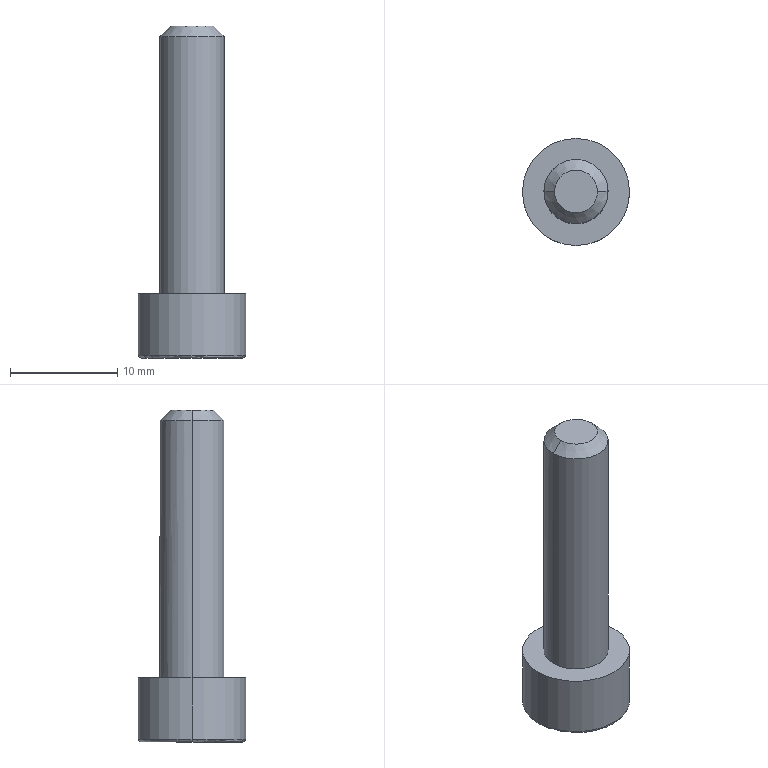Part | STEP file | Positioning_id2202_x_t | 1 solid | 18 faces | box 10 x 10 x 31 mm | volume 1106 mm3 | plane 10 | cylinder 4 | cone 2 | torus 2 | commonest cylinder face diameters 6 x2 10 x2
STEP:
#1=CARTESIAN_POINT('',(0.,0.,0.));
#2=DIRECTION('',(0.,0.,1.));
#3=DIRECTION('',(1.,0.,0.));
#4=AXIS2_PLACEMENT_3D('',#1,#2,#3);
#5=CARTESIAN_POINT('',(-1005.502,416.,55.5));
#6=VERTEX_POINT('',#5);
#7=CARTESIAN_POINT('',(-1004.502,416.,56.5));
#8=VERTEX_POINT('',#7);
#9=CARTESIAN_POINT('',(-1004.502,416.,56.5));
#10=DIRECTION('',(0.7071,0.,0.7071));
#11=VECTOR('',#10,1.);
#12=LINE('',#9,#11);
#13=CARTESIAN_POINT('',(-1002.502,416.,55.5));
#14=DIRECTION('',(0.,0.,-1.));
#15=DIRECTION('',(-1.,0.,0.));
#16=AXIS2_PLACEMENT_3D('',#13,#14,#15);
#17=CONICAL_SURFACE('',#16,3.,0.7854);
#18=CARTESIAN_POINT('',(0.,-1.));
#19=DIRECTION('',(0.,-1.));
#20=VECTOR('',#19,1.);
#21=LINE('',#18,#20);
#22=(GEOMETRIC_REPRESENTATION_CONTEXT(2)PARAMETRIC_REPRESENTATION_CONTEXT()REPRESENTATION_CONTEXT('',''));
#23=DEFINITIONAL_REPRESENTATION('',(#21),#22);
#24=PCURVE('',#17,#23);
#25=CARTESIAN_POINT('',(-1002.502,416.,55.5));
#26=DIRECTION('',(0.,0.,-1.));
#27=DIRECTION('',(-1.,0.,0.));
#28=AXIS2_PLACEMENT_3D('',#25,#26,#27);
#29=CONICAL_SURFACE('',#28,3.,0.7854);
#30=CARTESIAN_POINT('',(6.283,-1.));
#31=DIRECTION('',(0.,-1.));
#32=VECTOR('',#31,1.);
#33=LINE('',#30,#32);
#34=(GEOMETRIC_REPRESENTATION_CONTEXT(2)PARAMETRIC_REPRESENTATION_CONTEXT()REPRESENTATION_CONTEXT('',''));
#35=DEFINITIONAL_REPRESENTATION('',(#33),#34);
#36=PCURVE('',#29,#35);
#37=SURFACE_CURVE('',#12,(#24,#36),.PCURVE_S1.);
#38=EDGE_CURVE('',#6,#8,#37,.T.);
#39=ORIENTED_EDGE('',*,*,#38,.T.);
#40=CARTESIAN_POINT('',(-1000.502,416.,56.5));
#41=VERTEX_POINT('',#40);
#42=CARTESIAN_POINT('',(-1002.502,416.,56.5));
#43=DIRECTION('',(0.,0.,1.));
#44=DIRECTION('',(0.,1.,0.));
#45=AXIS2_PLACEMENT_3D('',#42,#43,#44);
#46=CIRCLE('',#45,2.);
#47=CARTESIAN_POINT('',(7.854,-1.));
#48=DIRECTION('',(-1.,0.));
#49=VECTOR('',#48,1.);
#50=LINE('',#47,#49);
#51=(GEOMETRIC_REPRESENTATION_CONTEXT(2)PARAMETRIC_REPRESENTATION_CONTEXT()REPRESENTATION_CONTEXT('',''));
#52=DEFINITIONAL_REPRESENTATION('',(#50),#51);
#53=PCURVE('',#17,#52);
#54=CARTESIAN_POINT('',(-1002.502,416.,56.5));
#55=DIRECTION('',(0.,0.,1.));
#56=DIRECTION('',(-1.,0.,0.));
#57=AXIS2_PLACEMENT_3D('',#54,#55,#56);
#58=PLANE('',#57);
#59=CARTESIAN_POINT('',(0.,0.));
#60=DIRECTION('',(0.,-1.));
#61=AXIS2_PLACEMENT_2D('',#59,#60);
#62=CIRCLE('',#61,2.);
#63=(GEOMETRIC_REPRESENTATION_CONTEXT(2)PARAMETRIC_REPRESENTATION_CONTEXT()REPRESENTATION_CONTEXT('',''));
#64=DEFINITIONAL_REPRESENTATION('',(#62),#63);
#65=PCURVE('',#58,#64);
#66=SURFACE_CURVE('',#46,(#53,#65),.PCURVE_S1.);
#67=EDGE_CURVE('',#41,#8,#66,.T.);
#68=ORIENTED_EDGE('',*,*,#67,.F.);
#69=CARTESIAN_POINT('',(-999.502,416.,55.5));
#70=VERTEX_POINT('',#69);
#71=CARTESIAN_POINT('',(-1000.502,416.,56.5));
#72=DIRECTION('',(0.7071,0.,-0.7071));
#73=VECTOR('',#72,1.);
#74=LINE('',#71,#73);
#75=CARTESIAN_POINT('',(3.142,-1.));
#76=DIRECTION('',(0.,1.));
#77=VECTOR('',#76,1.);
#78=LINE('',#75,#77);
#79=(GEOMETRIC_REPRESENTATION_CONTEXT(2)PARAMETRIC_REPRESENTATION_CONTEXT()REPRESENTATION_CONTEXT('',''));
#80=DEFINITIONAL_REPRESENTATION('',(#78),#79);
#81=PCURVE('',#17,#80);
#82=CARTESIAN_POINT('',(3.142,-1.));
#83=DIRECTION('',(0.,1.));
#84=VECTOR('',#83,1.);
#85=LINE('',#82,#84);
#86=(GEOMETRIC_REPRESENTATION_CONTEXT(2)PARAMETRIC_REPRESENTATION_CONTEXT()REPRESENTATION_CONTEXT('',''));
#87=DEFINITIONAL_REPRESENTATION('',(#85),#86);
#88=PCURVE('',#29,#87);
#89=SURFACE_CURVE('',#74,(#81,#88),.PCURVE_S1.);
#90=EDGE_CURVE('',#41,#70,#89,.T.);
#91=ORIENTED_EDGE('',*,*,#90,.T.);
#92=CARTESIAN_POINT('',(-1002.502,416.,55.5));
#93=DIRECTION('',(0.,0.,-1.));
#94=DIRECTION('',(-1.,0.,0.));
#95=AXIS2_PLACEMENT_3D('',#92,#93,#94);
#96=CIRCLE('',#95,3.);
#97=CARTESIAN_POINT('',(0.,0.));
#98=DIRECTION('',(1.,0.));
#99=VECTOR('',#98,1.);
#100=LINE('',#97,#99);
#101=(GEOMETRIC_REPRESENTATION_CONTEXT(2)PARAMETRIC_REPRESENTATION_CONTEXT()REPRESENTATION_CONTEXT('',''));
#102=DEFINITIONAL_REPRESENTATION('',(#100),#101);
#103=PCURVE('',#17,#102);
#104=CARTESIAN_POINT('',(-1002.502,416.,56.5));
#105=DIRECTION('',(0.,0.,1.));
#106=DIRECTION('',(1.,0.,0.));
#107=AXIS2_PLACEMENT_3D('',#104,#105,#106);
#108=CYLINDRICAL_SURFACE('',#107,3.);
#109=CARTESIAN_POINT('',(3.142,-1.));
#110=DIRECTION('',(-1.,0.));
#111=VECTOR('',#110,1.);
#112=LINE('',#109,#111);
#113=(GEOMETRIC_REPRESENTATION_CONTEXT(2)PARAMETRIC_REPRESENTATION_CONTEXT()REPRESENTATION_CONTEXT('',''));
#114=DEFINITIONAL_REPRESENTATION('',(#112),#113);
#115=PCURVE('',#108,#114);
#116=SURFACE_CURVE('',#96,(#103,#115),.PCURVE_S1.);
#117=EDGE_CURVE('',#6,#70,#116,.T.);
#118=ORIENTED_EDGE('',*,*,#117,.F.);
#119=EDGE_LOOP('',(#39,#68,#91,#118));
#120=FACE_BOUND('',#119,.T.);
#121=ADVANCED_FACE('',(#120),#17,.T.);
#122=CARTESIAN_POINT('',(-999.502,416.,31.5));
#123=VERTEX_POINT('',#122);
#124=CARTESIAN_POINT('',(-999.502,416.,55.5));
#125=DIRECTION('',(0.,0.,1.));
#126=VECTOR('',#125,1.);
#127=LINE('',#124,#126);
#128=CARTESIAN_POINT('',(-1002.502,416.,56.5));
#129=DIRECTION('',(0.,0.,1.));
#130=DIRECTION('',(1.,0.,0.));
#131=AXIS2_PLACEMENT_3D('',#128,#129,#130);
#132=CYLINDRICAL_SURFACE('',#131,3.);
#133=CARTESIAN_POINT('',(6.283,-1.));
#134=DIRECTION('',(0.,1.));
#135=VECTOR('',#134,1.);
#136=LINE('',#133,#135);
#137=(GEOMETRIC_REPRESENTATION_CONTEXT(2)PARAMETRIC_REPRESENTATION_CONTEXT()REPRESENTATION_CONTEXT('',''));
#138=DEFINITIONAL_REPRESENTATION('',(#136),#137);
#139=PCURVE('',#132,#138);
#140=CARTESIAN_POINT('',(0.,-1.));
#141=DIRECTION('',(0.,1.));
#142=VECTOR('',#141,1.);
#143=LINE('',#140,#142);
#144=(GEOMETRIC_REPRESENTATION_CONTEXT(2)PARAMETRIC_REPRESENTATION_CONTEXT()REPRESENTATION_CONTEXT('',''));
#145=DEFINITIONAL_REPRESENTATION('',(#143),#144);
#146=PCURVE('',#108,#145);
#147=SURFACE_CURVE('',#127,(#139,#146),.PCURVE_S1.);
#148=EDGE_CURVE('',#123,#70,#147,.T.);
#149=ORIENTED_EDGE('',*,*,#148,.T.);
#150=CARTESIAN_POINT('',(-1002.502,416.,55.5));
#151=DIRECTION('',(0.,0.,-1.));
#152=DIRECTION('',(1.,0.,0.));
#153=AXIS2_PLACEMENT_3D('',#150,#151,#152);
#154=CIRCLE('',#153,3.);
#155=CARTESIAN_POINT('',(6.283,-1.));
#156=DIRECTION('',(-1.,0.));
#157=VECTOR('',#156,1.);
#158=LINE('',#155,#157);
#159=(GEOMETRIC_REPRESENTATION_CONTEXT(2)PARAMETRIC_REPRESENTATION_CONTEXT()REPRESENTATION_CONTEXT('',''));
#160=DEFINITIONAL_REPRESENTATION('',(#158),#159);
#161=PCURVE('',#132,#160);
#162=CARTESIAN_POINT('',(3.142,0.));
#163=DIRECTION('',(1.,0.));
#164=VECTOR('',#163,1.);
#165=LINE('',#162,#164);
#166=(GEOMETRIC_REPRESENTATION_CONTEXT(2)PARAMETRIC_REPRESENTATION_CONTEXT()REPRESENTATION_CONTEXT('',''));
#167=DEFINITIONAL_REPRESENTATION('',(#165),#166);
#168=PCURVE('',#29,#167);
#169=SURFACE_CURVE('',#154,(#161,#168),.PCURVE_S1.);
#170=EDGE_CURVE('',#70,#6,#169,.T.);
#171=ORIENTED_EDGE('',*,*,#170,.T.);
#172=CARTESIAN_POINT('',(-1005.502,416.,31.5));
#173=VERTEX_POINT('',#172);
#174=CARTESIAN_POINT('',(-1005.502,416.,55.5));
#175=DIRECTION('',(0.,0.,-1.));
#176=VECTOR('',#175,1.);
#177=LINE('',#174,#176);
#178=CARTESIAN_POINT('',(3.142,-1.));
#179=DIRECTION('',(0.,-1.));
#180=VECTOR('',#179,1.);
#181=LINE('',#178,#180);
#182=(GEOMETRIC_REPRESENTATION_CONTEXT(2)PARAMETRIC_REPRESENTATION_CONTEXT()REPRESENTATION_CONTEXT('',''));
#183=DEFINITIONAL_REPRESENTATION('',(#181),#182);
#184=PCURVE('',#132,#183);
#185=CARTESIAN_POINT('',(3.142,-1.));
#186=DIRECTION('',(0.,-1.));
#187=VECTOR('',#186,1.);
#188=LINE('',#185,#187);
#189=(GEOMETRIC_REPRESENTATION_CONTEXT(2)PARAMETRIC_REPRESENTATION_CONTEXT()REPRESENTATION_CONTEXT('',''));
#190=DEFINITIONAL_REPRESENTATION('',(#188),#189);
#191=PCURVE('',#108,#190);
#192=SURFACE_CURVE('',#177,(#184,#191),.PCURVE_S1.);
#193=EDGE_CURVE('',#6,#173,#192,.T.);
#194=ORIENTED_EDGE('',*,*,#193,.T.);
#195=CARTESIAN_POINT('',(-1002.502,416.,31.5));
#196=DIRECTION('',(0.,0.,1.));
#197=DIRECTION('',(0.,-1.,0.));
#198=AXIS2_PLACEMENT_3D('',#195,#196,#197);
#199=CIRCLE('',#198,3.);
#200=CARTESIAN_POINT('',(-1.571,-25.));
#201=DIRECTION('',(1.,0.));
#202=VECTOR('',#201,1.);
#203=LINE('',#200,#202);
#204=(GEOMETRIC_REPRESENTATION_CONTEXT(2)PARAMETRIC_REPRESENTATION_CONTEXT()REPRESENTATION_CONTEXT('',''));
#205=DEFINITIONAL_REPRESENTATION('',(#203),#204);
#206=PCURVE('',#132,#205);
#207=CARTESIAN_POINT('',(-1002.502,411.,31.5));
#208=DIRECTION('',(0.,0.,1.));
#209=DIRECTION('',(-1.,0.,0.));
#210=AXIS2_PLACEMENT_3D('',#207,#208,#209);
#211=PLANE('',#210);
#212=CARTESIAN_POINT('',(0.,-5.));
#213=DIRECTION('',(0.,1.));
#214=AXIS2_PLACEMENT_2D('',#212,#213);
#215=CIRCLE('',#214,3.);
#216=(GEOMETRIC_REPRESENTATION_CONTEXT(2)PARAMETRIC_REPRESENTATION_CONTEXT()REPRESENTATION_CONTEXT('',''));
#217=DEFINITIONAL_REPRESENTATION('',(#215),#216);
#218=PCURVE('',#211,#217);
#219=SURFACE_CURVE('',#199,(#206,#218),.PCURVE_S1.);
#220=EDGE_CURVE('',#173,#123,#219,.T.);
#221=ORIENTED_EDGE('',*,*,#220,.T.);
#222=EDGE_LOOP('',(#149,#171,#194,#221));
#223=FACE_BOUND('',#222,.T.);
#224=ADVANCED_FACE('',(#223),#132,.T.);
#225=ORIENTED_EDGE('',*,*,#67,.T.);
#226=CARTESIAN_POINT('',(-1004.502,416.,56.5));
#227=CARTESIAN_POINT('',(-1004.502,414.,56.5));
#228=CARTESIAN_POINT('',(-1002.502,413.,56.5));
#229=CARTESIAN_POINT('',(-1000.502,414.,56.5));
#230=CARTESIAN_POINT('',(-1000.502,416.,56.5));
#231=(BOUNDED_CURVE()B_SPLINE_CURVE(4,(#226,#227,#228,#229,#230),.UNSPECIFIED.,.F.,.F.)B_SPLINE_CURVE_WITH_KNOTS((5,5),(0.,1.),.PIECEWISE_BEZIER_KNOTS.)CURVE()GEOMETRIC_REPRESENTATION_ITEM()RATIONAL_B_SPLINE_CURVE((1.,0.7071,0.6667,0.7071,1.))REPRESENTATION_ITEM(''));
#232=CARTESIAN_POINT('',(2.,0.));
#233=CARTESIAN_POINT('',(2.,2.));
#234=CARTESIAN_POINT('',(0.,3.));
#235=CARTESIAN_POINT('',(-2.,2.));
#236=CARTESIAN_POINT('',(-2.,0.));
#237=(BOUNDED_CURVE()B_SPLINE_CURVE(4,(#232,#233,#234,#235,#236),.UNSPECIFIED.,.F.,.F.)B_SPLINE_CURVE_WITH_KNOTS((5,5),(0.,1.),.PIECEWISE_BEZIER_KNOTS.)CURVE()GEOMETRIC_REPRESENTATION_ITEM()RATIONAL_B_SPLINE_CURVE((1.,0.7071,0.6667,0.7071,1.))REPRESENTATION_ITEM(''));
#238=(GEOMETRIC_REPRESENTATION_CONTEXT(2)PARAMETRIC_REPRESENTATION_CONTEXT()REPRESENTATION_CONTEXT('',''));
#239=DEFINITIONAL_REPRESENTATION('',(#237),#238);
#240=PCURVE('',#58,#239);
#241=CARTESIAN_POINT('',(6.283,-1.));
#242=CARTESIAN_POINT('',(6.24,-1.));
#243=CARTESIAN_POINT('',(6.153,-1.));
#244=CARTESIAN_POINT('',(6.02,-1.));
#245=CARTESIAN_POINT('',(5.883,-1.));
#246=CARTESIAN_POINT('',(5.744,-1.));
#247=CARTESIAN_POINT('',(5.602,-1.));
#248=CARTESIAN_POINT('',(5.457,-1.));
#249=CARTESIAN_POINT('',(5.311,-1.));
#250=CARTESIAN_POINT('',(5.163,-1.));
#251=CARTESIAN_POINT('',(5.013,-1.));
#252=CARTESIAN_POINT('',(4.863,-1.));
#253=CARTESIAN_POINT('',(4.712,-1.));
#254=CARTESIAN_POINT('',(4.562,-1.));
#255=CARTESIAN_POINT('',(4.412,-1.));
#256=CARTESIAN_POINT('',(4.262,-1.));
#257=CARTESIAN_POINT('',(4.114,-1.));
#258=CARTESIAN_POINT('',(3.968,-1.));
#259=CARTESIAN_POINT('',(3.823,-1.));
#260=CARTESIAN_POINT('',(3.681,-1.));
#261=CARTESIAN_POINT('',(3.542,-1.));
#262=CARTESIAN_POINT('',(3.405,-1.));
#263=CARTESIAN_POINT('',(3.271,-1.));
#264=CARTESIAN_POINT('',(3.184,-1.));
#265=CARTESIAN_POINT('',(3.142,-1.));
#266=B_SPLINE_CURVE_WITH_KNOTS('',3,(#241,#242,#243,#244,#245,#246,#247,#248,#249,#250,#251,#252,#253,#254,#255,#256,#257,#258,#259,#260,#261,#262,#263,#264,#265),.UNSPECIFIED.,.F.,.F.,(4,1,1,1,1,1,1,1,1,1,1,1,1,1,1,1,1,1,1,1,1,1,4),(0.,0.04545,0.09091,0.1364,0.1818,0.2273,0.2727,0.3182,0.3636,0.4091,0.4545,0.5,0.5455,0.5909,0.6364,0.6818,0.7273,0.7727,0.8182,0.8636,0.9091,0.9545,1.),.QUASI_UNIFORM_KNOTS.);
#267=(GEOMETRIC_REPRESENTATION_CONTEXT(2)PARAMETRIC_REPRESENTATION_CONTEXT()REPRESENTATION_CONTEXT('',''));
#268=DEFINITIONAL_REPRESENTATION('',(#266),#267);
#269=PCURVE('',#29,#268);
#270=SURFACE_CURVE('',#231,(#240,#269),.PCURVE_S1.);
#271=EDGE_CURVE('',#8,#41,#270,.T.);
#272=ORIENTED_EDGE('',*,*,#271,.T.);
#273=EDGE_LOOP('',(#225,#272));
#274=FACE_BOUND('',#273,.T.);
#275=ADVANCED_FACE('',(#274),#58,.T.);
#276=ORIENTED_EDGE('',*,*,#220,.F.);
#277=CARTESIAN_POINT('',(-1002.502,419.,31.5));
#278=VERTEX_POINT('',#277);
#279=CARTESIAN_POINT('',(-1002.502,419.,31.5));
#280=CARTESIAN_POINT('',(-1005.502,419.,31.5));
#281=CARTESIAN_POINT('',(-1005.502,416.,31.5));
#282=(BOUNDED_CURVE()B_SPLINE_CURVE(2,(#279,#280,#281),.UNSPECIFIED.,.F.,.F.)B_SPLINE_CURVE_WITH_KNOTS((3,3),(0.,1.),.PIECEWISE_BEZIER_KNOTS.)CURVE()GEOMETRIC_REPRESENTATION_ITEM()RATIONAL_B_SPLINE_CURVE((1.,0.7071,1.))REPRESENTATION_ITEM(''));
#283=CARTESIAN_POINT('',(0.,-8.));
#284=CARTESIAN_POINT('',(3.,-8.));
#285=CARTESIAN_POINT('',(3.,-5.));
#286=(BOUNDED_CURVE()B_SPLINE_CURVE(2,(#283,#284,#285),.UNSPECIFIED.,.F.,.F.)B_SPLINE_CURVE_WITH_KNOTS((3,3),(0.,1.),.PIECEWISE_BEZIER_KNOTS.)CURVE()GEOMETRIC_REPRESENTATION_ITEM()RATIONAL_B_SPLINE_CURVE((1.,0.7071,1.))REPRESENTATION_ITEM(''));
#287=(GEOMETRIC_REPRESENTATION_CONTEXT(2)PARAMETRIC_REPRESENTATION_CONTEXT()REPRESENTATION_CONTEXT('',''));
#288=DEFINITIONAL_REPRESENTATION('',(#286),#287);
#289=PCURVE('',#211,#288);
#290=CARTESIAN_POINT('',(1.571,-25.));
#291=CARTESIAN_POINT('',(1.592,-25.));
#292=CARTESIAN_POINT('',(1.636,-25.));
#293=CARTESIAN_POINT('',(1.702,-25.));
#294=CARTESIAN_POINT('',(1.771,-25.));
#295=CARTESIAN_POINT('',(1.841,-25.));
#296=CARTESIAN_POINT('',(1.912,-25.));
#297=CARTESIAN_POINT('',(1.984,-25.));
#298=CARTESIAN_POINT('',(2.057,-25.));
#299=CARTESIAN_POINT('',(2.131,-25.));
#300=CARTESIAN_POINT('',(2.206,-25.));
#301=CARTESIAN_POINT('',(2.281,-25.));
#302=CARTESIAN_POINT('',(2.356,-25.));
#303=CARTESIAN_POINT('',(2.432,-25.));
#304=CARTESIAN_POINT('',(2.507,-25.));
#305=CARTESIAN_POINT('',(2.581,-25.));
#306=CARTESIAN_POINT('',(2.655,-25.));
#307=CARTESIAN_POINT('',(2.729,-25.));
#308=CARTESIAN_POINT('',(2.801,-25.));
#309=CARTESIAN_POINT('',(2.872,-25.));
#310=CARTESIAN_POINT('',(2.942,-25.));
#311=CARTESIAN_POINT('',(3.01,-25.));
#312=CARTESIAN_POINT('',(3.077,-25.));
#313=CARTESIAN_POINT('',(3.12,-25.));
#314=CARTESIAN_POINT('',(3.142,-25.));
#315=B_SPLINE_CURVE_WITH_KNOTS('',3,(#290,#291,#292,#293,#294,#295,#296,#297,#298,#299,#300,#301,#302,#303,#304,#305,#306,#307,#308,#309,#310,#311,#312,#313,#314),.UNSPECIFIED.,.F.,.F.,(4,1,1,1,1,1,1,1,1,1,1,1,1,1,1,1,1,1,1,1,1,1,4),(0.,0.04545,0.09091,0.1364,0.1818,0.2273,0.2727,0.3182,0.3636,0.4091,0.4545,0.5,0.5455,0.5909,0.6364,0.6818,0.7273,0.7727,0.8182,0.8636,0.9091,0.9545,1.),.QUASI_UNIFORM_KNOTS.);
#316=(GEOMETRIC_REPRESENTATION_CONTEXT(2)PARAMETRIC_REPRESENTATION_CONTEXT()REPRESENTATION_CONTEXT('',''));
#317=DEFINITIONAL_REPRESENTATION('',(#315),#316);
#318=PCURVE('',#108,#317);
#319=SURFACE_CURVE('',#282,(#289,#318),.PCURVE_S1.);
#320=EDGE_CURVE('',#278,#173,#319,.T.);
#321=ORIENTED_EDGE('',*,*,#320,.F.);
#322=CARTESIAN_POINT('',(-999.502,416.,31.5));
#323=CARTESIAN_POINT('',(-999.502,419.,31.5));
#324=CARTESIAN_POINT('',(-1002.502,419.,31.5));
#325=(BOUNDED_CURVE()B_SPLINE_CURVE(2,(#322,#323,#324),.UNSPECIFIED.,.F.,.F.)B_SPLINE_CURVE_WITH_KNOTS((3,3),(0.,1.),.PIECEWISE_BEZIER_KNOTS.)CURVE()GEOMETRIC_REPRESENTATION_ITEM()RATIONAL_B_SPLINE_CURVE((1.,0.7071,1.))REPRESENTATION_ITEM(''));
#326=CARTESIAN_POINT('',(-3.,-5.));
#327=CARTESIAN_POINT('',(-3.,-8.));
#328=CARTESIAN_POINT('',(0.,-8.));
#329=(BOUNDED_CURVE()B_SPLINE_CURVE(2,(#326,#327,#328),.UNSPECIFIED.,.F.,.F.)B_SPLINE_CURVE_WITH_KNOTS((3,3),(0.,1.),.PIECEWISE_BEZIER_KNOTS.)CURVE()GEOMETRIC_REPRESENTATION_ITEM()RATIONAL_B_SPLINE_CURVE((1.,0.7071,1.))REPRESENTATION_ITEM(''));
#330=(GEOMETRIC_REPRESENTATION_CONTEXT(2)PARAMETRIC_REPRESENTATION_CONTEXT()REPRESENTATION_CONTEXT('',''));
#331=DEFINITIONAL_REPRESENTATION('',(#329),#330);
#332=PCURVE('',#211,#331);
#333=CARTESIAN_POINT('',(0.,-25.));
#334=CARTESIAN_POINT('',(0.02143,-25.));
#335=CARTESIAN_POINT('',(0.06485,-25.));
#336=CARTESIAN_POINT('',(0.1316,-25.));
#337=CARTESIAN_POINT('',(0.2,-25.));
#338=CARTESIAN_POINT('',(0.2697,-25.));
#339=CARTESIAN_POINT('',(0.3408,-25.));
#340=CARTESIAN_POINT('',(0.413,-25.));
#341=CARTESIAN_POINT('',(0.4863,-25.));
#342=CARTESIAN_POINT('',(0.5603,-25.));
#343=CARTESIAN_POINT('',(0.635,-25.));
#344=CARTESIAN_POINT('',(0.7101,-25.));
#345=CARTESIAN_POINT('',(0.7854,-25.));
#346=CARTESIAN_POINT('',(0.8607,-25.));
#347=CARTESIAN_POINT('',(0.9358,-25.));
#348=CARTESIAN_POINT('',(1.01,-25.));
#349=CARTESIAN_POINT('',(1.085,-25.));
#350=CARTESIAN_POINT('',(1.158,-25.));
#351=CARTESIAN_POINT('',(1.23,-25.));
#352=CARTESIAN_POINT('',(1.301,-25.));
#353=CARTESIAN_POINT('',(1.371,-25.));
#354=CARTESIAN_POINT('',(1.439,-25.));
#355=CARTESIAN_POINT('',(1.506,-25.));
#356=CARTESIAN_POINT('',(1.549,-25.));
#357=CARTESIAN_POINT('',(1.571,-25.));
#358=B_SPLINE_CURVE_WITH_KNOTS('',3,(#333,#334,#335,#336,#337,#338,#339,#340,#341,#342,#343,#344,#345,#346,#347,#348,#349,#350,#351,#352,#353,#354,#355,#356,#357),.UNSPECIFIED.,.F.,.F.,(4,1,1,1,1,1,1,1,1,1,1,1,1,1,1,1,1,1,1,1,1,1,4),(0.,0.04545,0.09091,0.1364,0.1818,0.2273,0.2727,0.3182,0.3636,0.4091,0.4545,0.5,0.5455,0.5909,0.6364,0.6818,0.7273,0.7727,0.8182,0.8636,0.9091,0.9545,1.),.QUASI_UNIFORM_KNOTS.);
#359=(GEOMETRIC_REPRESENTATION_CONTEXT(2)PARAMETRIC_REPRESENTATION_CONTEXT()REPRESENTATION_CONTEXT('',''));
#360=DEFINITIONAL_REPRESENTATION('',(#358),#359);
#361=PCURVE('',#108,#360);
#362=SURFACE_CURVE('',#325,(#332,#361),.PCURVE_S1.);
#363=EDGE_CURVE('',#123,#278,#362,.T.);
#364=ORIENTED_EDGE('',*,*,#363,.F.);
#365=EDGE_LOOP('',(#276,#321,#364));
#366=FACE_BOUND('',#365,.T.);
#367=CARTESIAN_POINT('',(-1007.502,416.,31.5));
#368=VERTEX_POINT('',#367);
#369=CARTESIAN_POINT('',(-997.502,416.,31.5));
#370=VERTEX_POINT('',#369);
#371=CARTESIAN_POINT('',(-1002.502,416.,31.5));
#372=DIRECTION('',(0.,0.,1.));
#373=DIRECTION('',(-1.,0.,0.));
#374=AXIS2_PLACEMENT_3D('',#371,#372,#373);
#375=CIRCLE('',#374,5.);
#376=CARTESIAN_POINT('',(0.,-5.));
#377=DIRECTION('',(1.,0.));
#378=AXIS2_PLACEMENT_2D('',#376,#377);
#379=CIRCLE('',#378,5.);
#380=(GEOMETRIC_REPRESENTATION_CONTEXT(2)PARAMETRIC_REPRESENTATION_CONTEXT()REPRESENTATION_CONTEXT('',''));
#381=DEFINITIONAL_REPRESENTATION('',(#379),#380);
#382=PCURVE('',#211,#381);
#383=CARTESIAN_POINT('',(-1002.502,416.,31.5));
#384=DIRECTION('',(0.,0.,1.));
#385=DIRECTION('',(1.,0.,0.));
#386=AXIS2_PLACEMENT_3D('',#383,#384,#385);
#387=CYLINDRICAL_SURFACE('',#386,5.);
#388=CARTESIAN_POINT('',(3.142,0.));
#389=DIRECTION('',(1.,0.));
#390=VECTOR('',#389,1.);
#391=LINE('',#388,#390);
#392=(GEOMETRIC_REPRESENTATION_CONTEXT(2)PARAMETRIC_REPRESENTATION_CONTEXT()REPRESENTATION_CONTEXT('',''));
#393=DEFINITIONAL_REPRESENTATION('',(#391),#392);
#394=PCURVE('',#387,#393);
#395=SURFACE_CURVE('',#375,(#382,#394),.PCURVE_S1.);
#396=EDGE_CURVE('',#368,#370,#395,.T.);
#397=ORIENTED_EDGE('',*,*,#396,.T.);
#398=CARTESIAN_POINT('',(-1002.502,416.,31.5));
#399=DIRECTION('',(0.,0.,1.));
#400=DIRECTION('',(1.,0.,0.));
#401=AXIS2_PLACEMENT_3D('',#398,#399,#400);
#402=CIRCLE('',#401,5.);
#403=CARTESIAN_POINT('',(0.,-5.));
#404=DIRECTION('',(-1.,0.));
#405=AXIS2_PLACEMENT_2D('',#403,#404);
#406=CIRCLE('',#405,5.);
#407=(GEOMETRIC_REPRESENTATION_CONTEXT(2)PARAMETRIC_REPRESENTATION_CONTEXT()REPRESENTATION_CONTEXT('',''));
#408=DEFINITIONAL_REPRESENTATION('',(#406),#407);
#409=PCURVE('',#211,#408);
#410=CARTESIAN_POINT('',(-1002.502,416.,31.5));
#411=DIRECTION('',(0.,0.,1.));
#412=DIRECTION('',(1.,0.,0.));
#413=AXIS2_PLACEMENT_3D('',#410,#411,#412);
#414=CYLINDRICAL_SURFACE('',#413,5.);
#415=CARTESIAN_POINT('',(0.,0.));
#416=DIRECTION('',(1.,0.));
#417=VECTOR('',#416,1.);
#418=LINE('',#415,#417);
#419=(GEOMETRIC_REPRESENTATION_CONTEXT(2)PARAMETRIC_REPRESENTATION_CONTEXT()REPRESENTATION_CONTEXT('',''));
#420=DEFINITIONAL_REPRESENTATION('',(#418),#419);
#421=PCURVE('',#414,#420);
#422=SURFACE_CURVE('',#402,(#409,#421),.PCURVE_S1.);
#423=EDGE_CURVE('',#370,#368,#422,.T.);
#424=ORIENTED_EDGE('',*,*,#423,.T.);
#425=EDGE_LOOP('',(#397,#424));
#426=FACE_BOUND('',#425,.T.);
#427=ADVANCED_FACE('',(#366,#426),#211,.T.);
#428=CARTESIAN_POINT('',(-997.502,416.,25.75));
#429=VERTEX_POINT('',#428);
#430=CARTESIAN_POINT('',(-997.502,416.,31.5));
#431=DIRECTION('',(0.,0.,-1.));
#432=VECTOR('',#431,1.);
#433=LINE('',#430,#432);
#434=CARTESIAN_POINT('',(6.283,0.));
#435=DIRECTION('',(0.,-1.));
#436=VECTOR('',#435,1.);
#437=LINE('',#434,#436);
#438=(GEOMETRIC_REPRESENTATION_CONTEXT(2)PARAMETRIC_REPRESENTATION_CONTEXT()REPRESENTATION_CONTEXT('',''));
#439=DEFINITIONAL_REPRESENTATION('',(#437),#438);
#440=PCURVE('',#387,#439);
#441=CARTESIAN_POINT('',(0.,0.));
#442=DIRECTION('',(0.,-1.));
#443=VECTOR('',#442,1.);
#444=LINE('',#441,#443);
#445=(GEOMETRIC_REPRESENTATION_CONTEXT(2)PARAMETRIC_REPRESENTATION_CONTEXT()REPRESENTATION_CONTEXT('',''));
#446=DEFINITIONAL_REPRESENTATION('',(#444),#445);
#447=PCURVE('',#414,#446);
#448=SURFACE_CURVE('',#433,(#440,#447),.PCURVE_S1.);
#449=EDGE_CURVE('',#370,#429,#448,.T.);
#450=ORIENTED_EDGE('',*,*,#449,.F.);
#451=ORIENTED_EDGE('',*,*,#396,.F.);
#452=CARTESIAN_POINT('',(-1007.502,416.,25.75));
#453=VERTEX_POINT('',#452);
#454=CARTESIAN_POINT('',(-1007.502,416.,31.5));
#455=DIRECTION('',(0.,0.,1.));
#456=VECTOR('',#455,1.);
#457=LINE('',#454,#456);
#458=CARTESIAN_POINT('',(3.142,0.));
#459=DIRECTION('',(0.,1.));
#460=VECTOR('',#459,1.);
#461=LINE('',#458,#460);
#462=(GEOMETRIC_REPRESENTATION_CONTEXT(2)PARAMETRIC_REPRESENTATION_CONTEXT()REPRESENTATION_CONTEXT('',''));
#463=DEFINITIONAL_REPRESENTATION('',(#461),#462);
#464=PCURVE('',#387,#463);
#465=CARTESIAN_POINT('',(3.142,0.));
#466=DIRECTION('',(0.,1.));
#467=VECTOR('',#466,1.);
#468=LINE('',#465,#467);
#469=(GEOMETRIC_REPRESENTATION_CONTEXT(2)PARAMETRIC_REPRESENTATION_CONTEXT()REPRESENTATION_CONTEXT('',''));
#470=DEFINITIONAL_REPRESENTATION('',(#468),#469);
#471=PCURVE('',#414,#470);
#472=SURFACE_CURVE('',#457,(#464,#471),.PCURVE_S1.);
#473=EDGE_CURVE('',#453,#368,#472,.T.);
#474=ORIENTED_EDGE('',*,*,#473,.F.);
#475=CARTESIAN_POINT('',(-1002.502,416.,25.75));
#476=DIRECTION('',(0.,0.,1.));
#477=DIRECTION('',(-1.,0.,0.));
#478=AXIS2_PLACEMENT_3D('',#475,#476,#477);
#479=CIRCLE('',#478,5.);
#480=CARTESIAN_POINT('',(3.142,-5.75));
#481=DIRECTION('',(1.,0.));
#482=VECTOR('',#481,1.);
#483=LINE('',#480,#482);
#484=(GEOMETRIC_REPRESENTATION_CONTEXT(2)PARAMETRIC_REPRESENTATION_CONTEXT()REPRESENTATION_CONTEXT('',''));
#485=DEFINITIONAL_REPRESENTATION('',(#483),#484);
#486=PCURVE('',#387,#485);
#487=CARTESIAN_POINT('',(-1002.502,416.,25.75));
#488=DIRECTION('',(0.,0.,-1.));
#489=DIRECTION('',(1.,0.,0.));
#490=AXIS2_PLACEMENT_3D('',#487,#488,#489);
#491=TOROIDAL_SURFACE('',#490,4.75,0.25);
#492=CARTESIAN_POINT('',(3.142,0.));
#493=DIRECTION('',(-1.,0.));
#494=VECTOR('',#493,1.);
#495=LINE('',#492,#494);
#496=(GEOMETRIC_REPRESENTATION_CONTEXT(2)PARAMETRIC_REPRESENTATION_CONTEXT()REPRESENTATION_CONTEXT('',''));
#497=DEFINITIONAL_REPRESENTATION('',(#495),#496);
#498=PCURVE('',#491,#497);
#499=SURFACE_CURVE('',#479,(#486,#498),.PCURVE_S1.);
#500=EDGE_CURVE('',#453,#429,#499,.T.);
#501=ORIENTED_EDGE('',*,*,#500,.T.);
#502=EDGE_LOOP('',(#450,#451,#474,#501));
#503=FACE_BOUND('',#502,.T.);
#504=ADVANCED_FACE('',(#503),#387,.T.);
#505=CARTESIAN_POINT('',(-997.752,416.,25.5));
#506=VERTEX_POINT('',#505);
#507=CARTESIAN_POINT('',(-997.752,416.,25.75));
#508=DIRECTION('',(0.,1.,0.));
#509=DIRECTION('',(1.,0.,0.));
#510=AXIS2_PLACEMENT_3D('',#507,#508,#509);
#511=CIRCLE('',#510,0.25);
#512=CARTESIAN_POINT('',(0.,0.));
#513=DIRECTION('',(0.,1.));
#514=VECTOR('',#513,1.);
#515=LINE('',#512,#514);
#516=(GEOMETRIC_REPRESENTATION_CONTEXT(2)PARAMETRIC_REPRESENTATION_CONTEXT()REPRESENTATION_CONTEXT('',''));
#517=DEFINITIONAL_REPRESENTATION('',(#515),#516);
#518=PCURVE('',#491,#517);
#519=CARTESIAN_POINT('',(-1002.502,416.,25.75));
#520=DIRECTION('',(0.,0.,-1.));
#521=DIRECTION('',(1.,0.,0.));
#522=AXIS2_PLACEMENT_3D('',#519,#520,#521);
#523=TOROIDAL_SURFACE('',#522,4.75,0.25);
#524=CARTESIAN_POINT('',(6.283,0.));
#525=DIRECTION('',(0.,1.));
#526=VECTOR('',#525,1.);
#527=LINE('',#524,#526);
#528=(GEOMETRIC_REPRESENTATION_CONTEXT(2)PARAMETRIC_REPRESENTATION_CONTEXT()REPRESENTATION_CONTEXT('',''));
#529=DEFINITIONAL_REPRESENTATION('',(#527),#528);
#530=PCURVE('',#523,#529);
#531=SURFACE_CURVE('',#511,(#518,#530),.PCURVE_S1.);
#532=EDGE_CURVE('',#429,#506,#531,.T.);
#533=ORIENTED_EDGE('',*,*,#532,.F.);
#534=ORIENTED_EDGE('',*,*,#500,.F.);
#535=CARTESIAN_POINT('',(-1007.252,416.,25.5));
#536=VERTEX_POINT('',#535);
#537=CARTESIAN_POINT('',(-1007.252,416.,25.75));
#538=DIRECTION('',(0.,1.,0.));
#539=DIRECTION('',(-1.,0.,0.));
#540=AXIS2_PLACEMENT_3D('',#537,#538,#539);
#541=CIRCLE('',#540,0.25);
#542=CARTESIAN_POINT('',(3.142,6.283));
#543=DIRECTION('',(0.,-1.));
#544=VECTOR('',#543,1.);
#545=LINE('',#542,#544);
#546=(GEOMETRIC_REPRESENTATION_CONTEXT(2)PARAMETRIC_REPRESENTATION_CONTEXT()REPRESENTATION_CONTEXT('',''));
#547=DEFINITIONAL_REPRESENTATION('',(#545),#546);
#548=PCURVE('',#491,#547);
#549=CARTESIAN_POINT('',(3.142,6.283));
#550=DIRECTION('',(0.,-1.));
#551=VECTOR('',#550,1.);
#552=LINE('',#549,#551);
#553=(GEOMETRIC_REPRESENTATION_CONTEXT(2)PARAMETRIC_REPRESENTATION_CONTEXT()REPRESENTATION_CONTEXT('',''));
#554=DEFINITIONAL_REPRESENTATION('',(#552),#553);
#555=PCURVE('',#523,#554);
#556=SURFACE_CURVE('',#541,(#548,#555),.PCURVE_S1.);
#557=EDGE_CURVE('',#536,#453,#556,.T.);
#558=ORIENTED_EDGE('',*,*,#557,.F.);
#559=CARTESIAN_POINT('',(-1007.252,416.,25.5));
#560=CARTESIAN_POINT('',(-1007.252,415.352,25.5));
#561=CARTESIAN_POINT('',(-1006.994,414.109,25.5));
#562=CARTESIAN_POINT('',(-1005.911,412.517,25.5));
#563=CARTESIAN_POINT('',(-1004.341,411.487,25.5));
#564=CARTESIAN_POINT('',(-1002.45,411.126,25.5));
#565=CARTESIAN_POINT('',(-1000.611,411.508,25.5));
#566=CARTESIAN_POINT('',(-999.019,412.591,25.5));
#567=CARTESIAN_POINT('',(-997.988,414.161,25.5));
#568=CARTESIAN_POINT('',(-997.752,415.404,25.5));
#569=CARTESIAN_POINT('',(-997.752,416.,25.5));
#570=B_SPLINE_CURVE_WITH_KNOTS('',3,(#559,#560,#561,#562,#563,#564,#565,#566,#567,#568,#569),.UNSPECIFIED.,.F.,.F.,(4,1,1,1,1,1,1,1,4),(0.,0.1302,0.25,0.3802,0.5,0.6302,0.75,0.8802,1.),.UNSPECIFIED.);
#571=CARTESIAN_POINT('',(3.142,1.571));
#572=CARTESIAN_POINT('',(3.118,1.571));
#573=CARTESIAN_POINT('',(3.07,1.571));
#574=CARTESIAN_POINT('',(2.999,1.572));
#575=CARTESIAN_POINT('',(2.927,1.572));
#576=CARTESIAN_POINT('',(2.856,1.572));
#577=CARTESIAN_POINT('',(2.785,1.571));
#578=CARTESIAN_POINT('',(2.713,1.57));
#579=CARTESIAN_POINT('',(2.642,1.571));
#580=CARTESIAN_POINT('',(2.57,1.571));
#581=CARTESIAN_POINT('',(2.499,1.571));
#582=CARTESIAN_POINT('',(2.428,1.57));
#583=CARTESIAN_POINT('',(2.356,1.57));
#584=CARTESIAN_POINT('',(2.285,1.571));
#585=CARTESIAN_POINT('',(2.213,1.572));
#586=CARTESIAN_POINT('',(2.142,1.572));
#587=CARTESIAN_POINT('',(2.071,1.571));
#588=CARTESIAN_POINT('',(1.999,1.57));
#589=CARTESIAN_POINT('',(1.928,1.57));
#590=CARTESIAN_POINT('',(1.856,1.571));
#591=CARTESIAN_POINT('',(1.785,1.571));
#592=CARTESIAN_POINT('',(1.714,1.571));
#593=CARTESIAN_POINT('',(1.642,1.57));
#594=CARTESIAN_POINT('',(1.571,1.57));
#595=CARTESIAN_POINT('',(1.499,1.571));
#596=CARTESIAN_POINT('',(1.428,1.572));
#597=CARTESIAN_POINT('',(1.357,1.572));
#598=CARTESIAN_POINT('',(1.285,1.571));
#599=CARTESIAN_POINT('',(1.214,1.57));
#600=CARTESIAN_POINT('',(1.142,1.57));
#601=CARTESIAN_POINT('',(1.071,1.57));
#602=CARTESIAN_POINT('',(0.9996,1.571));
#603=CARTESIAN_POINT('',(0.9282,1.571));
#604=CARTESIAN_POINT('',(0.8568,1.57));
#605=CARTESIAN_POINT('',(0.7854,1.57));
#606=CARTESIAN_POINT('',(0.714,1.571));
#607=CARTESIAN_POINT('',(0.6426,1.572));
#608=CARTESIAN_POINT('',(0.5712,1.572));
#609=CARTESIAN_POINT('',(0.4998,1.571));
#610=CARTESIAN_POINT('',(0.4284,1.57));
#611=CARTESIAN_POINT('',(0.357,1.57));
#612=CARTESIAN_POINT('',(0.2856,1.571));
#613=CARTESIAN_POINT('',(0.2142,1.571));
#614=CARTESIAN_POINT('',(0.1428,1.571));
#615=CARTESIAN_POINT('',(0.0714,1.571));
#616=CARTESIAN_POINT('',(0.0238,1.571));
#617=CARTESIAN_POINT('',(0.,1.571));
#618=B_SPLINE_CURVE_WITH_KNOTS('',3,(#571,#572,#573,#574,#575,#576,#577,#578,#579,#580,#581,#582,#583,#584,#585,#586,#587,#588,#589,#590,#591,#592,#593,#594,#595,#596,#597,#598,#599,#600,#601,#602,#603,#604,#605,#606,#607,#608,#609,#610,#611,#612,#613,#614,#615,#616,#617),.UNSPECIFIED.,.F.,.F.,(4,1,1,1,1,1,1,1,1,1,1,1,1,1,1,1,1,1,1,1,1,1,1,1,1,1,1,1,1,1,1,1,1,1,1,1,1,1,1,1,1,1,1,1,4),(0.,0.02273,0.04545,0.06818,0.09091,0.1136,0.1364,0.1591,0.1818,0.2045,0.2273,0.25,0.2727,0.2955,0.3182,0.3409,0.3636,0.3864,0.4091,0.4318,0.4545,0.4773,0.5,0.5227,0.5455,0.5682,0.5909,0.6136,0.6364,0.6591,0.6818,0.7045,0.7273,0.75,0.7727,0.7955,0.8182,0.8409,0.8636,0.8864,0.9091,0.9318,0.9545,0.9773,1.),.QUASI_UNIFORM_KNOTS.);
#619=(GEOMETRIC_REPRESENTATION_CONTEXT(2)PARAMETRIC_REPRESENTATION_CONTEXT()REPRESENTATION_CONTEXT('',''));
#620=DEFINITIONAL_REPRESENTATION('',(#618),#619);
#621=PCURVE('',#491,#620);
#622=CARTESIAN_POINT('',(-1002.502,416.,25.5));
#623=DIRECTION('',(0.,0.,-1.));
#624=DIRECTION('',(1.,0.,0.));
#625=AXIS2_PLACEMENT_3D('',#622,#623,#624);
#626=PLANE('',#625);
#627=CARTESIAN_POINT('',(-4.75,0.));
#628=CARTESIAN_POINT('',(-4.75,0.6477));
#629=CARTESIAN_POINT('',(-4.492,1.891));
#630=CARTESIAN_POINT('',(-3.409,3.483));
#631=CARTESIAN_POINT('',(-1.839,4.513));
#632=CARTESIAN_POINT('',(0.05196,4.874));
#633=CARTESIAN_POINT('',(1.891,4.492));
#634=CARTESIAN_POINT('',(3.483,3.409));
#635=CARTESIAN_POINT('',(4.514,1.839));
#636=CARTESIAN_POINT('',(4.75,0.5958));
#637=CARTESIAN_POINT('',(4.75,0.));
#638=B_SPLINE_CURVE_WITH_KNOTS('',3,(#627,#628,#629,#630,#631,#632,#633,#634,#635,#636,#637),.UNSPECIFIED.,.F.,.F.,(4,1,1,1,1,1,1,1,4),(0.,0.1302,0.25,0.3802,0.5,0.6302,0.75,0.8802,1.),.UNSPECIFIED.);
#639=(GEOMETRIC_REPRESENTATION_CONTEXT(2)PARAMETRIC_REPRESENTATION_CONTEXT()REPRESENTATION_CONTEXT('',''));
#640=DEFINITIONAL_REPRESENTATION('',(#638),#639);
#641=PCURVE('',#626,#640);
#642=SURFACE_CURVE('',#570,(#621,#641),.PCURVE_S1.);
#643=EDGE_CURVE('',#536,#506,#642,.T.);
#644=ORIENTED_EDGE('',*,*,#643,.T.);
#645=EDGE_LOOP('',(#533,#534,#558,#644));
#646=FACE_BOUND('',#645,.T.);
#647=ADVANCED_FACE('',(#646),#491,.T.);
#648=CARTESIAN_POINT('',(-1002.502,418.86,25.5));
#649=VERTEX_POINT('',#648);
#650=CARTESIAN_POINT('',(-1000.025,417.43,25.5));
#651=VERTEX_POINT('',#650);
#652=CARTESIAN_POINT('',(-1002.502,418.86,25.5));
#653=DIRECTION('',(0.866,-0.5,0.));
#654=VECTOR('',#653,1.);
#655=LINE('',#652,#654);
#656=CARTESIAN_POINT('',(0.,-2.86));
#657=DIRECTION('',(0.866,0.5));
#658=VECTOR('',#657,1.);
#659=LINE('',#656,#658);
#660=(GEOMETRIC_REPRESENTATION_CONTEXT(2)PARAMETRIC_REPRESENTATION_CONTEXT()REPRESENTATION_CONTEXT('',''));
#661=DEFINITIONAL_REPRESENTATION('',(#659),#660);
#662=PCURVE('',#626,#661);
#663=CARTESIAN_POINT('',(-1002.502,418.86,28.5));
#664=DIRECTION('',(-0.5,-0.866,0.));
#665=DIRECTION('',(0.866,-0.5,0.));
#666=AXIS2_PLACEMENT_3D('',#663,#664,#665);
#667=PLANE('',#666);
#668=CARTESIAN_POINT('',(0.,-3.));
#669=DIRECTION('',(1.,0.));
#670=VECTOR('',#669,1.);
#671=LINE('',#668,#670);
#672=(GEOMETRIC_REPRESENTATION_CONTEXT(2)PARAMETRIC_REPRESENTATION_CONTEXT()REPRESENTATION_CONTEXT('',''));
#673=DEFINITIONAL_REPRESENTATION('',(#671),#672);
#674=PCURVE('',#667,#673);
#675=SURFACE_CURVE('',#655,(#662,#674),.PCURVE_S1.);
#676=EDGE_CURVE('',#649,#651,#675,.T.);
#677=ORIENTED_EDGE('',*,*,#676,.F.);
#678=CARTESIAN_POINT('',(-1004.979,417.43,25.5));
#679=VERTEX_POINT('',#678);
#680=CARTESIAN_POINT('',(-1004.979,417.43,25.5));
#681=DIRECTION('',(0.866,0.5,0.));
#682=VECTOR('',#681,1.);
#683=LINE('',#680,#682);
#684=CARTESIAN_POINT('',(-2.477,-1.43));
#685=DIRECTION('',(0.866,-0.5));
#686=VECTOR('',#685,1.);
#687=LINE('',#684,#686);
#688=(GEOMETRIC_REPRESENTATION_CONTEXT(2)PARAMETRIC_REPRESENTATION_CONTEXT()REPRESENTATION_CONTEXT('',''));
#689=DEFINITIONAL_REPRESENTATION('',(#687),#688);
#690=PCURVE('',#626,#689);
#691=CARTESIAN_POINT('',(-1004.979,417.43,28.5));
#692=DIRECTION('',(0.5,-0.866,0.));
#693=DIRECTION('',(0.866,0.5,0.));
#694=AXIS2_PLACEMENT_3D('',#691,#692,#693);
#695=PLANE('',#694);
#696=CARTESIAN_POINT('',(0.,-3.));
#697=DIRECTION('',(1.,0.));
#698=VECTOR('',#697,1.);
#699=LINE('',#696,#698);
#700=(GEOMETRIC_REPRESENTATION_CONTEXT(2)PARAMETRIC_REPRESENTATION_CONTEXT()REPRESENTATION_CONTEXT('',''));
#701=DEFINITIONAL_REPRESENTATION('',(#699),#700);
#702=PCURVE('',#695,#701);
#703=SURFACE_CURVE('',#683,(#690,#702),.PCURVE_S1.);
#704=EDGE_CURVE('',#679,#649,#703,.T.);
#705=ORIENTED_EDGE('',*,*,#704,.F.);
#706=CARTESIAN_POINT('',(-1004.979,414.57,25.5));
#707=VERTEX_POINT('',#706);
#708=CARTESIAN_POINT('',(-1004.979,414.57,25.5));
#709=DIRECTION('',(0.,1.,0.));
#710=VECTOR('',#709,1.);
#711=LINE('',#708,#710);
#712=CARTESIAN_POINT('',(-2.477,1.43));
#713=DIRECTION('',(0.,-1.));
#714=VECTOR('',#713,1.);
#715=LINE('',#712,#714);
#716=(GEOMETRIC_REPRESENTATION_CONTEXT(2)PARAMETRIC_REPRESENTATION_CONTEXT()REPRESENTATION_CONTEXT('',''));
#717=DEFINITIONAL_REPRESENTATION('',(#715),#716);
#718=PCURVE('',#626,#717);
#719=CARTESIAN_POINT('',(-1004.979,414.57,28.5));
#720=DIRECTION('',(1.,0.,0.));
#721=DIRECTION('',(0.,1.,0.));
#722=AXIS2_PLACEMENT_3D('',#719,#720,#721);
#723=PLANE('',#722);
#724=CARTESIAN_POINT('',(0.,-3.));
#725=DIRECTION('',(1.,0.));
#726=VECTOR('',#725,1.);
#727=LINE('',#724,#726);
#728=(GEOMETRIC_REPRESENTATION_CONTEXT(2)PARAMETRIC_REPRESENTATION_CONTEXT()REPRESENTATION_CONTEXT('',''));
#729=DEFINITIONAL_REPRESENTATION('',(#727),#728);
#730=PCURVE('',#723,#729);
#731=SURFACE_CURVE('',#711,(#718,#730),.PCURVE_S1.);
#732=EDGE_CURVE('',#707,#679,#731,.T.);
#733=ORIENTED_EDGE('',*,*,#732,.F.);
#734=CARTESIAN_POINT('',(-1002.502,413.14,25.5));
#735=VERTEX_POINT('',#734);
#736=CARTESIAN_POINT('',(-1002.502,413.14,25.5));
#737=DIRECTION('',(-0.866,0.5,0.));
#738=VECTOR('',#737,1.);
#739=LINE('',#736,#738);
#740=CARTESIAN_POINT('',(0.,2.86));
#741=DIRECTION('',(-0.866,-0.5));
#742=VECTOR('',#741,1.);
#743=LINE('',#740,#742);
#744=(GEOMETRIC_REPRESENTATION_CONTEXT(2)PARAMETRIC_REPRESENTATION_CONTEXT()REPRESENTATION_CONTEXT('',''));
#745=DEFINITIONAL_REPRESENTATION('',(#743),#744);
#746=PCURVE('',#626,#745);
#747=CARTESIAN_POINT('',(-1002.502,413.14,28.5));
#748=DIRECTION('',(0.5,0.866,0.));
#749=DIRECTION('',(-0.866,0.5,0.));
#750=AXIS2_PLACEMENT_3D('',#747,#748,#749);
#751=PLANE('',#750);
#752=CARTESIAN_POINT('',(0.,-3.));
#753=DIRECTION('',(1.,0.));
#754=VECTOR('',#753,1.);
#755=LINE('',#752,#754);
#756=(GEOMETRIC_REPRESENTATION_CONTEXT(2)PARAMETRIC_REPRESENTATION_CONTEXT()REPRESENTATION_CONTEXT('',''));
#757=DEFINITIONAL_REPRESENTATION('',(#755),#756);
#758=PCURVE('',#751,#757);
#759=SURFACE_CURVE('',#739,(#746,#758),.PCURVE_S1.);
#760=EDGE_CURVE('',#735,#707,#759,.T.);
#761=ORIENTED_EDGE('',*,*,#760,.F.);
#762=CARTESIAN_POINT('',(-1000.025,414.57,25.5));
#763=VERTEX_POINT('',#762);
#764=CARTESIAN_POINT('',(-1000.025,414.57,25.5));
#765=DIRECTION('',(-0.866,-0.5,0.));
#766=VECTOR('',#765,1.);
#767=LINE('',#764,#766);
#768=CARTESIAN_POINT('',(2.477,1.43));
#769=DIRECTION('',(-0.866,0.5));
#770=VECTOR('',#769,1.);
#771=LINE('',#768,#770);
#772=(GEOMETRIC_REPRESENTATION_CONTEXT(2)PARAMETRIC_REPRESENTATION_CONTEXT()REPRESENTATION_CONTEXT('',''));
#773=DEFINITIONAL_REPRESENTATION('',(#771),#772);
#774=PCURVE('',#626,#773);
#775=CARTESIAN_POINT('',(-1000.025,414.57,28.5));
#776=DIRECTION('',(-0.5,0.866,0.));
#777=DIRECTION('',(-0.866,-0.5,0.));
#778=AXIS2_PLACEMENT_3D('',#775,#776,#777);
#779=PLANE('',#778);
#780=CARTESIAN_POINT('',(0.,-3.));
#781=DIRECTION('',(1.,0.));
#782=VECTOR('',#781,1.);
#783=LINE('',#780,#782);
#784=(GEOMETRIC_REPRESENTATION_CONTEXT(2)PARAMETRIC_REPRESENTATION_CONTEXT()REPRESENTATION_CONTEXT('',''));
#785=DEFINITIONAL_REPRESENTATION('',(#783),#784);
#786=PCURVE('',#779,#785);
#787=SURFACE_CURVE('',#767,(#774,#786),.PCURVE_S1.);
#788=EDGE_CURVE('',#763,#735,#787,.T.);
#789=ORIENTED_EDGE('',*,*,#788,.F.);
#790=CARTESIAN_POINT('',(-1000.025,417.43,25.5));
#791=DIRECTION('',(0.,-1.,0.));
#792=VECTOR('',#791,1.);
#793=LINE('',#790,#792);
#794=CARTESIAN_POINT('',(2.477,-1.43));
#795=DIRECTION('',(0.,1.));
#796=VECTOR('',#795,1.);
#797=LINE('',#794,#796);
#798=(GEOMETRIC_REPRESENTATION_CONTEXT(2)PARAMETRIC_REPRESENTATION_CONTEXT()REPRESENTATION_CONTEXT('',''));
#799=DEFINITIONAL_REPRESENTATION('',(#797),#798);
#800=PCURVE('',#626,#799);
#801=CARTESIAN_POINT('',(-1000.025,417.43,28.5));
#802=DIRECTION('',(-1.,0.,0.));
#803=DIRECTION('',(0.,-1.,0.));
#804=AXIS2_PLACEMENT_3D('',#801,#802,#803);
#805=PLANE('',#804);
#806=CARTESIAN_POINT('',(0.,-3.));
#807=DIRECTION('',(1.,0.));
#808=VECTOR('',#807,1.);
#809=LINE('',#806,#808);
#810=(GEOMETRIC_REPRESENTATION_CONTEXT(2)PARAMETRIC_REPRESENTATION_CONTEXT()REPRESENTATION_CONTEXT('',''));
#811=DEFINITIONAL_REPRESENTATION('',(#809),#810);
#812=PCURVE('',#805,#811);
#813=SURFACE_CURVE('',#793,(#800,#812),.PCURVE_S1.);
#814=EDGE_CURVE('',#651,#763,#813,.T.);
#815=ORIENTED_EDGE('',*,*,#814,.F.);
#816=EDGE_LOOP('',(#677,#705,#733,#761,#789,#815));
#817=FACE_BOUND('',#816,.T.);
#818=ORIENTED_EDGE('',*,*,#643,.F.);
#819=CARTESIAN_POINT('',(-1002.502,416.,25.5));
#820=DIRECTION('',(0.,0.,1.));
#821=DIRECTION('',(1.,0.,0.));
#822=AXIS2_PLACEMENT_3D('',#819,#820,#821);
#823=CIRCLE('',#822,4.75);
#824=CARTESIAN_POINT('',(4.75,0.));
#825=CARTESIAN_POINT('',(4.75,-8.227));
#826=CARTESIAN_POINT('',(-2.375,-4.114));
#827=CARTESIAN_POINT('',(-9.5,0.));
#828=CARTESIAN_POINT('',(-2.375,4.114));
#829=CARTESIAN_POINT('',(4.75,8.227));
#830=CARTESIAN_POINT('',(4.75,0.));
#831=(BOUNDED_CURVE()B_SPLINE_CURVE(2,(#824,#825,#826,#827,#828,#829,#830),.UNSPECIFIED.,.T.,.F.)B_SPLINE_CURVE_WITH_KNOTS((1,2,2,2,2,1),(-2.094,0.,2.094,4.189,6.283,8.378),.UNSPECIFIED.)CURVE()GEOMETRIC_REPRESENTATION_ITEM()RATIONAL_B_SPLINE_CURVE((1.,0.5,1.,0.5,1.,0.5,1.))REPRESENTATION_ITEM(''));
#832=(GEOMETRIC_REPRESENTATION_CONTEXT(2)PARAMETRIC_REPRESENTATION_CONTEXT()REPRESENTATION_CONTEXT('',''));
#833=DEFINITIONAL_REPRESENTATION('',(#831),#832);
#834=PCURVE('',#626,#833);
#835=CARTESIAN_POINT('',(6.283,1.571));
#836=DIRECTION('',(-1.,0.));
#837=VECTOR('',#836,1.);
#838=LINE('',#835,#837);
#839=(GEOMETRIC_REPRESENTATION_CONTEXT(2)PARAMETRIC_REPRESENTATION_CONTEXT()REPRESENTATION_CONTEXT('',''));
#840=DEFINITIONAL_REPRESENTATION('',(#838),#839);
#841=PCURVE('',#523,#840);
#842=SURFACE_CURVE('',#823,(#834,#841),.PCURVE_S1.);
#843=EDGE_CURVE('',#506,#536,#842,.T.);
#844=ORIENTED_EDGE('',*,*,#843,.F.);
#845=EDGE_LOOP('',(#818,#844));
#846=FACE_BOUND('',#845,.T.);
#847=ADVANCED_FACE('',(#817,#846),#626,.T.);
#848=CARTESIAN_POINT('',(-1002.502,418.86,28.5));
#849=VERTEX_POINT('',#848);
#850=CARTESIAN_POINT('',(-1000.025,417.43,28.5));
#851=VERTEX_POINT('',#850);
#852=CARTESIAN_POINT('',(-1002.502,418.86,28.5));
#853=DIRECTION('',(0.866,-0.5,0.));
#854=VECTOR('',#853,1.);
#855=LINE('',#852,#854);
#856=CARTESIAN_POINT('',(0.,0.));
#857=DIRECTION('',(1.,0.));
#858=VECTOR('',#857,1.);
#859=LINE('',#856,#858);
#860=(GEOMETRIC_REPRESENTATION_CONTEXT(2)PARAMETRIC_REPRESENTATION_CONTEXT()REPRESENTATION_CONTEXT('',''));
#861=DEFINITIONAL_REPRESENTATION('',(#859),#860);
#862=PCURVE('',#667,#861);
#863=CARTESIAN_POINT('',(-1000.025,414.57,28.5));
#864=DIRECTION('',(0.,0.,1.));
#865=DIRECTION('',(0.,1.,0.));
#866=AXIS2_PLACEMENT_3D('',#863,#864,#865);
#867=PLANE('',#866);
#868=CARTESIAN_POINT('',(4.29,2.477));
#869=DIRECTION('',(-0.5,-0.866));
#870=VECTOR('',#869,1.);
#871=LINE('',#868,#870);
#872=(GEOMETRIC_REPRESENTATION_CONTEXT(2)PARAMETRIC_REPRESENTATION_CONTEXT()REPRESENTATION_CONTEXT('',''));
#873=DEFINITIONAL_REPRESENTATION('',(#871),#872);
#874=PCURVE('',#867,#873);
#875=SURFACE_CURVE('',#855,(#862,#874),.PCURVE_S1.);
#876=EDGE_CURVE('',#849,#851,#875,.T.);
#877=ORIENTED_EDGE('',*,*,#876,.F.);
#878=CARTESIAN_POINT('',(-1002.502,418.86,28.5));
#879=DIRECTION('',(0.,0.,-1.));
#880=VECTOR('',#879,1.);
#881=LINE('',#878,#880);
#882=CARTESIAN_POINT('',(0.,0.));
#883=DIRECTION('',(0.,-1.));
#884=VECTOR('',#883,1.);
#885=LINE('',#882,#884);
#886=(GEOMETRIC_REPRESENTATION_CONTEXT(2)PARAMETRIC_REPRESENTATION_CONTEXT()REPRESENTATION_CONTEXT('',''));
#887=DEFINITIONAL_REPRESENTATION('',(#885),#886);
#888=PCURVE('',#667,#887);
#889=CARTESIAN_POINT('',(2.86,0.));
#890=DIRECTION('',(0.,-1.));
#891=VECTOR('',#890,1.);
#892=LINE('',#889,#891);
#893=(GEOMETRIC_REPRESENTATION_CONTEXT(2)PARAMETRIC_REPRESENTATION_CONTEXT()REPRESENTATION_CONTEXT('',''));
#894=DEFINITIONAL_REPRESENTATION('',(#892),#893);
#895=PCURVE('',#695,#894);
#896=SURFACE_CURVE('',#881,(#888,#895),.PCURVE_S1.);
#897=EDGE_CURVE('',#849,#649,#896,.T.);
#898=ORIENTED_EDGE('',*,*,#897,.T.);
#899=ORIENTED_EDGE('',*,*,#676,.T.);
#900=CARTESIAN_POINT('',(-1000.025,417.43,28.5));
#901=DIRECTION('',(0.,0.,-1.));
#902=VECTOR('',#901,1.);
#903=LINE('',#900,#902);
#904=CARTESIAN_POINT('',(2.86,0.));
#905=DIRECTION('',(0.,-1.));
#906=VECTOR('',#905,1.);
#907=LINE('',#904,#906);
#908=(GEOMETRIC_REPRESENTATION_CONTEXT(2)PARAMETRIC_REPRESENTATION_CONTEXT()REPRESENTATION_CONTEXT('',''));
#909=DEFINITIONAL_REPRESENTATION('',(#907),#908);
#910=PCURVE('',#667,#909);
#911=CARTESIAN_POINT('',(0.,0.));
#912=DIRECTION('',(0.,-1.));
#913=VECTOR('',#912,1.);
#914=LINE('',#911,#913);
#915=(GEOMETRIC_REPRESENTATION_CONTEXT(2)PARAMETRIC_REPRESENTATION_CONTEXT()REPRESENTATION_CONTEXT('',''));
#916=DEFINITIONAL_REPRESENTATION('',(#914),#915);
#917=PCURVE('',#805,#916);
#918=SURFACE_CURVE('',#903,(#910,#917),.PCURVE_S1.);
#919=EDGE_CURVE('',#851,#651,#918,.T.);
#920=ORIENTED_EDGE('',*,*,#919,.F.);
#921=EDGE_LOOP('',(#877,#898,#899,#920));
#922=FACE_BOUND('',#921,.T.);
#923=ADVANCED_FACE('',(#922),#667,.T.);
#924=CARTESIAN_POINT('',(-1000.025,414.57,28.5));
#925=VERTEX_POINT('',#924);
#926=CARTESIAN_POINT('',(-1000.025,414.57,28.5));
#927=DIRECTION('',(0.,0.,-1.));
#928=VECTOR('',#927,1.);
#929=LINE('',#926,#928);
#930=CARTESIAN_POINT('',(2.86,0.));
#931=DIRECTION('',(0.,-1.));
#932=VECTOR('',#931,1.);
#933=LINE('',#930,#932);
#934=(GEOMETRIC_REPRESENTATION_CONTEXT(2)PARAMETRIC_REPRESENTATION_CONTEXT()REPRESENTATION_CONTEXT('',''));
#935=DEFINITIONAL_REPRESENTATION('',(#933),#934);
#936=PCURVE('',#805,#935);
#937=CARTESIAN_POINT('',(0.,0.));
#938=DIRECTION('',(0.,-1.));
#939=VECTOR('',#938,1.);
#940=LINE('',#937,#939);
#941=(GEOMETRIC_REPRESENTATION_CONTEXT(2)PARAMETRIC_REPRESENTATION_CONTEXT()REPRESENTATION_CONTEXT('',''));
#942=DEFINITIONAL_REPRESENTATION('',(#940),#941);
#943=PCURVE('',#779,#942);
#944=SURFACE_CURVE('',#929,(#936,#943),.PCURVE_S1.);
#945=EDGE_CURVE('',#925,#763,#944,.T.);
#946=ORIENTED_EDGE('',*,*,#945,.F.);
#947=CARTESIAN_POINT('',(-1000.025,417.43,28.5));
#948=DIRECTION('',(0.,-1.,0.));
#949=VECTOR('',#948,1.);
#950=LINE('',#947,#949);
#951=CARTESIAN_POINT('',(0.,0.));
#952=DIRECTION('',(1.,0.));
#953=VECTOR('',#952,1.);
#954=LINE('',#951,#953);
#955=(GEOMETRIC_REPRESENTATION_CONTEXT(2)PARAMETRIC_REPRESENTATION_CONTEXT()REPRESENTATION_CONTEXT('',''));
#956=DEFINITIONAL_REPRESENTATION('',(#954),#955);
#957=PCURVE('',#805,#956);
#958=CARTESIAN_POINT('',(2.86,0.));
#959=DIRECTION('',(-1.,0.));
#960=VECTOR('',#959,1.);
#961=LINE('',#958,#960);
#962=(GEOMETRIC_REPRESENTATION_CONTEXT(2)PARAMETRIC_REPRESENTATION_CONTEXT()REPRESENTATION_CONTEXT('',''));
#963=DEFINITIONAL_REPRESENTATION('',(#961),#962);
#964=PCURVE('',#867,#963);
#965=SURFACE_CURVE('',#950,(#957,#964),.PCURVE_S1.);
#966=EDGE_CURVE('',#851,#925,#965,.T.);
#967=ORIENTED_EDGE('',*,*,#966,.F.);
#968=ORIENTED_EDGE('',*,*,#919,.T.);
#969=ORIENTED_EDGE('',*,*,#814,.T.);
#970=EDGE_LOOP('',(#946,#967,#968,#969));
#971=FACE_BOUND('',#970,.T.);
#972=ADVANCED_FACE('',(#971),#805,.T.);
#973=CARTESIAN_POINT('',(-1002.502,413.14,28.5));
#974=VERTEX_POINT('',#973);
#975=CARTESIAN_POINT('',(-1002.502,413.14,28.5));
#976=DIRECTION('',(0.,0.,-1.));
#977=VECTOR('',#976,1.);
#978=LINE('',#975,#977);
#979=CARTESIAN_POINT('',(2.86,0.));
#980=DIRECTION('',(0.,-1.));
#981=VECTOR('',#980,1.);
#982=LINE('',#979,#981);
#983=(GEOMETRIC_REPRESENTATION_CONTEXT(2)PARAMETRIC_REPRESENTATION_CONTEXT()REPRESENTATION_CONTEXT('',''));
#984=DEFINITIONAL_REPRESENTATION('',(#982),#983);
#985=PCURVE('',#779,#984);
#986=CARTESIAN_POINT('',(0.,0.));
#987=DIRECTION('',(0.,-1.));
#988=VECTOR('',#987,1.);
#989=LINE('',#986,#988);
#990=(GEOMETRIC_REPRESENTATION_CONTEXT(2)PARAMETRIC_REPRESENTATION_CONTEXT()REPRESENTATION_CONTEXT('',''));
#991=DEFINITIONAL_REPRESENTATION('',(#989),#990);
#992=PCURVE('',#751,#991);
#993=SURFACE_CURVE('',#978,(#985,#992),.PCURVE_S1.);
#994=EDGE_CURVE('',#974,#735,#993,.T.);
#995=ORIENTED_EDGE('',*,*,#994,.F.);
#996=CARTESIAN_POINT('',(-1000.025,414.57,28.5));
#997=DIRECTION('',(-0.866,-0.5,0.));
#998=VECTOR('',#997,1.);
#999=LINE('',#996,#998);
#1000=CARTESIAN_POINT('',(0.,0.));
#1001=DIRECTION('',(1.,0.));
#1002=VECTOR('',#1001,1.);
#1003=LINE('',#1000,#1002);
#1004=(GEOMETRIC_REPRESENTATION_CONTEXT(2)PARAMETRIC_REPRESENTATION_CONTEXT()REPRESENTATION_CONTEXT('',''));
#1005=DEFINITIONAL_REPRESENTATION('',(#1003),#1004);
#1006=PCURVE('',#779,#1005);
#1007=CARTESIAN_POINT('',(0.,0.));
#1008=DIRECTION('',(-0.5,0.866));
#1009=VECTOR('',#1008,1.);
#1010=LINE('',#1007,#1009);
#1011=(GEOMETRIC_REPRESENTATION_CONTEXT(2)PARAMETRIC_REPRESENTATION_CONTEXT()REPRESENTATION_CONTEXT('',''));
#1012=DEFINITIONAL_REPRESENTATION('',(#1010),#1011);
#1013=PCURVE('',#867,#1012);
#1014=SURFACE_CURVE('',#999,(#1006,#1013),.PCURVE_S1.);
#1015=EDGE_CURVE('',#925,#974,#1014,.T.);
#1016=ORIENTED_EDGE('',*,*,#1015,.F.);
#1017=ORIENTED_EDGE('',*,*,#945,.T.);
#1018=ORIENTED_EDGE('',*,*,#788,.T.);
#1019=EDGE_LOOP('',(#995,#1016,#1017,#1018));
#1020=FACE_BOUND('',#1019,.T.);
#1021=ADVANCED_FACE('',(#1020),#779,.T.);
#1022=CARTESIAN_POINT('',(-1004.979,414.57,28.5));
#1023=VERTEX_POINT('',#1022);
#1024=CARTESIAN_POINT('',(-1004.979,414.57,28.5));
#1025=DIRECTION('',(0.,0.,-1.));
#1026=VECTOR('',#1025,1.);
#1027=LINE('',#1024,#1026);
#1028=CARTESIAN_POINT('',(2.86,0.));
#1029=DIRECTION('',(0.,-1.));
#1030=VECTOR('',#1029,1.);
#1031=LINE('',#1028,#1030);
#1032=(GEOMETRIC_REPRESENTATION_CONTEXT(2)PARAMETRIC_REPRESENTATION_CONTEXT()REPRESENTATION_CONTEXT('',''));
#1033=DEFINITIONAL_REPRESENTATION('',(#1031),#1032);
#1034=PCURVE('',#751,#1033);
#1035=CARTESIAN_POINT('',(0.,0.));
#1036=DIRECTION('',(0.,-1.));
#1037=VECTOR('',#1036,1.);
#1038=LINE('',#1035,#1037);
#1039=(GEOMETRIC_REPRESENTATION_CONTEXT(2)PARAMETRIC_REPRESENTATION_CONTEXT()REPRESENTATION_CONTEXT('',''));
#1040=DEFINITIONAL_REPRESENTATION('',(#1038),#1039);
#1041=PCURVE('',#723,#1040);
#1042=SURFACE_CURVE('',#1027,(#1034,#1041),.PCURVE_S1.);
#1043=EDGE_CURVE('',#1023,#707,#1042,.T.);
#1044=ORIENTED_EDGE('',*,*,#1043,.F.);
#1045=CARTESIAN_POINT('',(-1002.502,413.14,28.5));
#1046=DIRECTION('',(-0.866,0.5,0.));
#1047=VECTOR('',#1046,1.);
#1048=LINE('',#1045,#1047);
#1049=CARTESIAN_POINT('',(0.,0.));
#1050=DIRECTION('',(1.,0.));
#1051=VECTOR('',#1050,1.);
#1052=LINE('',#1049,#1051);
#1053=(GEOMETRIC_REPRESENTATION_CONTEXT(2)PARAMETRIC_REPRESENTATION_CONTEXT()REPRESENTATION_CONTEXT('',''));
#1054=DEFINITIONAL_REPRESENTATION('',(#1052),#1053);
#1055=PCURVE('',#751,#1054);
#1056=CARTESIAN_POINT('',(-1.43,2.477));
#1057=DIRECTION('',(0.5,0.866));
#1058=VECTOR('',#1057,1.);
#1059=LINE('',#1056,#1058);
#1060=(GEOMETRIC_REPRESENTATION_CONTEXT(2)PARAMETRIC_REPRESENTATION_CONTEXT()REPRESENTATION_CONTEXT('',''));
#1061=DEFINITIONAL_REPRESENTATION('',(#1059),#1060);
#1062=PCURVE('',#867,#1061);
#1063=SURFACE_CURVE('',#1048,(#1055,#1062),.PCURVE_S1.);
#1064=EDGE_CURVE('',#974,#1023,#1063,.T.);
#1065=ORIENTED_EDGE('',*,*,#1064,.F.);
#1066=ORIENTED_EDGE('',*,*,#994,.T.);
#1067=ORIENTED_EDGE('',*,*,#760,.T.);
#1068=EDGE_LOOP('',(#1044,#1065,#1066,#1067));
#1069=FACE_BOUND('',#1068,.T.);
#1070=ADVANCED_FACE('',(#1069),#751,.T.);
#1071=CARTESIAN_POINT('',(-1004.979,417.43,28.5));
#1072=VERTEX_POINT('',#1071);
#1073=CARTESIAN_POINT('',(-1004.979,417.43,28.5));
#1074=DIRECTION('',(0.,0.,-1.));
#1075=VECTOR('',#1074,1.);
#1076=LINE('',#1073,#1075);
#1077=CARTESIAN_POINT('',(2.86,0.));
#1078=DIRECTION('',(0.,-1.));
#1079=VECTOR('',#1078,1.);
#1080=LINE('',#1077,#1079);
#1081=(GEOMETRIC_REPRESENTATION_CONTEXT(2)PARAMETRIC_REPRESENTATION_CONTEXT()REPRESENTATION_CONTEXT('',''));
#1082=DEFINITIONAL_REPRESENTATION('',(#1080),#1081);
#1083=PCURVE('',#723,#1082);
#1084=CARTESIAN_POINT('',(0.,0.));
#1085=DIRECTION('',(0.,-1.));
#1086=VECTOR('',#1085,1.);
#1087=LINE('',#1084,#1086);
#1088=(GEOMETRIC_REPRESENTATION_CONTEXT(2)PARAMETRIC_REPRESENTATION_CONTEXT()REPRESENTATION_CONTEXT('',''));
#1089=DEFINITIONAL_REPRESENTATION('',(#1087),#1088);
#1090=PCURVE('',#695,#1089);
#1091=SURFACE_CURVE('',#1076,(#1083,#1090),.PCURVE_S1.);
#1092=EDGE_CURVE('',#1072,#679,#1091,.T.);
#1093=ORIENTED_EDGE('',*,*,#1092,.F.);
#1094=CARTESIAN_POINT('',(-1004.979,414.57,28.5));
#1095=DIRECTION('',(0.,1.,0.));
#1096=VECTOR('',#1095,1.);
#1097=LINE('',#1094,#1096);
#1098=CARTESIAN_POINT('',(0.,0.));
#1099=DIRECTION('',(1.,0.));
#1100=VECTOR('',#1099,1.);
#1101=LINE('',#1098,#1100);
#1102=(GEOMETRIC_REPRESENTATION_CONTEXT(2)PARAMETRIC_REPRESENTATION_CONTEXT()REPRESENTATION_CONTEXT('',''));
#1103=DEFINITIONAL_REPRESENTATION('',(#1101),#1102);
#1104=PCURVE('',#723,#1103);
#1105=CARTESIAN_POINT('',(0.,4.954));
#1106=DIRECTION('',(1.,0.));
#1107=VECTOR('',#1106,1.);
#1108=LINE('',#1105,#1107);
#1109=(GEOMETRIC_REPRESENTATION_CONTEXT(2)PARAMETRIC_REPRESENTATION_CONTEXT()REPRESENTATION_CONTEXT('',''));
#1110=DEFINITIONAL_REPRESENTATION('',(#1108),#1109);
#1111=PCURVE('',#867,#1110);
#1112=SURFACE_CURVE('',#1097,(#1104,#1111),.PCURVE_S1.);
#1113=EDGE_CURVE('',#1023,#1072,#1112,.T.);
#1114=ORIENTED_EDGE('',*,*,#1113,.F.);
#1115=ORIENTED_EDGE('',*,*,#1043,.T.);
#1116=ORIENTED_EDGE('',*,*,#732,.T.);
#1117=EDGE_LOOP('',(#1093,#1114,#1115,#1116));
#1118=FACE_BOUND('',#1117,.T.);
#1119=ADVANCED_FACE('',(#1118),#723,.T.);
#1120=ORIENTED_EDGE('',*,*,#897,.F.);
#1121=CARTESIAN_POINT('',(-1004.979,417.43,28.5));
#1122=DIRECTION('',(0.866,0.5,0.));
#1123=VECTOR('',#1122,1.);
#1124=LINE('',#1121,#1123);
#1125=CARTESIAN_POINT('',(0.,0.));
#1126=DIRECTION('',(1.,0.));
#1127=VECTOR('',#1126,1.);
#1128=LINE('',#1125,#1127);
#1129=(GEOMETRIC_REPRESENTATION_CONTEXT(2)PARAMETRIC_REPRESENTATION_CONTEXT()REPRESENTATION_CONTEXT('',''));
#1130=DEFINITIONAL_REPRESENTATION('',(#1128),#1129);
#1131=PCURVE('',#695,#1130);
#1132=CARTESIAN_POINT('',(2.86,4.954));
#1133=DIRECTION('',(0.5,-0.866));
#1134=VECTOR('',#1133,1.);
#1135=LINE('',#1132,#1134);
#1136=(GEOMETRIC_REPRESENTATION_CONTEXT(2)PARAMETRIC_REPRESENTATION_CONTEXT()REPRESENTATION_CONTEXT('',''));
#1137=DEFINITIONAL_REPRESENTATION('',(#1135),#1136);
#1138=PCURVE('',#867,#1137);
#1139=SURFACE_CURVE('',#1124,(#1131,#1138),.PCURVE_S1.);
#1140=EDGE_CURVE('',#1072,#849,#1139,.T.);
#1141=ORIENTED_EDGE('',*,*,#1140,.F.);
#1142=ORIENTED_EDGE('',*,*,#1092,.T.);
#1143=ORIENTED_EDGE('',*,*,#704,.T.);
#1144=EDGE_LOOP('',(#1120,#1141,#1142,#1143));
#1145=FACE_BOUND('',#1144,.T.);
#1146=ADVANCED_FACE('',(#1145),#695,.T.);
#1147=ORIENTED_EDGE('',*,*,#966,.T.);
#1148=ORIENTED_EDGE('',*,*,#1015,.T.);
#1149=ORIENTED_EDGE('',*,*,#1064,.T.);
#1150=ORIENTED_EDGE('',*,*,#1113,.T.);
#1151=ORIENTED_EDGE('',*,*,#1140,.T.);
#1152=ORIENTED_EDGE('',*,*,#876,.T.);
#1153=EDGE_LOOP('',(#1147,#1148,#1149,#1150,#1151,#1152));
#1154=FACE_BOUND('',#1153,.T.);
#1155=ADVANCED_FACE('',(#1154),#867,.F.);
#1156=CARTESIAN_POINT('',(-1002.502,416.,25.75));
#1157=DIRECTION('',(0.,0.,1.));
#1158=DIRECTION('',(1.,0.,0.));
#1159=AXIS2_PLACEMENT_3D('',#1156,#1157,#1158);
#1160=CIRCLE('',#1159,5.);
#1161=CARTESIAN_POINT('',(6.283,0.));
#1162=CARTESIAN_POINT('',(6.236,0.));
#1163=CARTESIAN_POINT('',(6.14,0.));
#1164=CARTESIAN_POINT('',(5.998,0.));
#1165=CARTESIAN_POINT('',(5.855,0.));
#1166=CARTESIAN_POINT('',(5.712,0.));
#1167=CARTESIAN_POINT('',(5.569,0.));
#1168=CARTESIAN_POINT('',(5.426,0.));
#1169=CARTESIAN_POINT('',(5.284,0.));
#1170=CARTESIAN_POINT('',(5.141,0.));
#1171=CARTESIAN_POINT('',(4.998,0.));
#1172=CARTESIAN_POINT('',(4.855,0.));
#1173=CARTESIAN_POINT('',(4.712,0.));
#1174=CARTESIAN_POINT('',(4.57,0.));
#1175=CARTESIAN_POINT('',(4.427,0.));
#1176=CARTESIAN_POINT('',(4.284,0.));
#1177=CARTESIAN_POINT('',(4.141,0.));
#1178=CARTESIAN_POINT('',(3.998,0.));
#1179=CARTESIAN_POINT('',(3.856,0.));
#1180=CARTESIAN_POINT('',(3.713,0.));
#1181=CARTESIAN_POINT('',(3.57,0.));
#1182=CARTESIAN_POINT('',(3.427,0.));
#1183=CARTESIAN_POINT('',(3.284,0.));
#1184=CARTESIAN_POINT('',(3.189,0.));
#1185=CARTESIAN_POINT('',(3.142,0.));
#1186=B_SPLINE_CURVE_WITH_KNOTS('',3,(#1161,#1162,#1163,#1164,#1165,#1166,#1167,#1168,#1169,#1170,#1171,#1172,#1173,#1174,#1175,#1176,#1177,#1178,#1179,#1180,#1181,#1182,#1183,#1184,#1185),.UNSPECIFIED.,.F.,.F.,(4,1,1,1,1,1,1,1,1,1,1,1,1,1,1,1,1,1,1,1,1,1,4),(0.,0.1428,0.2856,0.4284,0.5712,0.714,0.8568,0.9996,1.142,1.285,1.428,1.571,1.714,1.856,1.999,2.142,2.285,2.428,2.57,2.713,2.856,2.999,3.142),.QUASI_UNIFORM_KNOTS.);
#1187=(GEOMETRIC_REPRESENTATION_CONTEXT(2)PARAMETRIC_REPRESENTATION_CONTEXT()REPRESENTATION_CONTEXT('',''));
#1188=DEFINITIONAL_REPRESENTATION('',(#1186),#1187);
#1189=PCURVE('',#523,#1188);
#1190=CARTESIAN_POINT('',(0.,-5.75));
#1191=DIRECTION('',(1.,0.));
#1192=VECTOR('',#1191,1.);
#1193=LINE('',#1190,#1192);
#1194=(GEOMETRIC_REPRESENTATION_CONTEXT(2)PARAMETRIC_REPRESENTATION_CONTEXT()REPRESENTATION_CONTEXT('',''));
#1195=DEFINITIONAL_REPRESENTATION('',(#1193),#1194);
#1196=PCURVE('',#414,#1195);
#1197=SURFACE_CURVE('',#1160,(#1189,#1196),.PCURVE_S1.);
#1198=EDGE_CURVE('',#429,#453,#1197,.T.);
#1199=ORIENTED_EDGE('',*,*,#1198,.F.);
#1200=ORIENTED_EDGE('',*,*,#532,.T.);
#1201=ORIENTED_EDGE('',*,*,#843,.T.);
#1202=ORIENTED_EDGE('',*,*,#557,.T.);
#1203=EDGE_LOOP('',(#1199,#1200,#1201,#1202));
#1204=FACE_BOUND('',#1203,.T.);
#1205=ADVANCED_FACE('',(#1204),#523,.T.);
#1206=ORIENTED_EDGE('',*,*,#423,.F.);
#1207=ORIENTED_EDGE('',*,*,#449,.T.);
#1208=ORIENTED_EDGE('',*,*,#1198,.T.);
#1209=ORIENTED_EDGE('',*,*,#473,.T.);
#1210=EDGE_LOOP('',(#1206,#1207,#1208,#1209));
#1211=FACE_BOUND('',#1210,.T.);
#1212=ADVANCED_FACE('',(#1211),#414,.T.);
#1213=ORIENTED_EDGE('',*,*,#117,.T.);
#1214=ORIENTED_EDGE('',*,*,#148,.F.);
#1215=ORIENTED_EDGE('',*,*,#363,.T.);
#1216=ORIENTED_EDGE('',*,*,#320,.T.);
#1217=ORIENTED_EDGE('',*,*,#193,.F.);
#1218=EDGE_LOOP('',(#1213,#1214,#1215,#1216,#1217));
#1219=FACE_BOUND('',#1218,.T.);
#1220=ADVANCED_FACE('',(#1219),#108,.T.);
#1221=ORIENTED_EDGE('',*,*,#271,.F.);
#1222=ORIENTED_EDGE('',*,*,#38,.F.);
#1223=ORIENTED_EDGE('',*,*,#170,.F.);
#1224=ORIENTED_EDGE('',*,*,#90,.F.);
#1225=EDGE_LOOP('',(#1221,#1222,#1223,#1224));
#1226=FACE_BOUND('',#1225,.T.);
#1227=ADVANCED_FACE('',(#1226),#29,.T.);
#1228=CLOSED_SHELL('',(#121,#224,#275,#427,#504,#647,#847,#923,#972,#1021,#1070,#1119,#1146,#1155,#1205,#1212,#1220,#1227));
#1229=MANIFOLD_SOLID_BREP('',#1228);
#1230=(LENGTH_UNIT()NAMED_UNIT(*)SI_UNIT(.MILLI.,.METRE.));
#1231=UNCERTAINTY_MEASURE_WITH_UNIT(LENGTH_MEASURE(0.0000001),#1230,'','');
#1232=(NAMED_UNIT(*)PLANE_ANGLE_UNIT()SI_UNIT($,.RADIAN.));
#1233=(NAMED_UNIT(*)SI_UNIT($,.STERADIAN.)SOLID_ANGLE_UNIT());
#1234=(GEOMETRIC_REPRESENTATION_CONTEXT(3)GLOBAL_UNCERTAINTY_ASSIGNED_CONTEXT((#1231))GLOBAL_UNIT_ASSIGNED_CONTEXT((#1230,#1232,#1233))REPRESENTATION_CONTEXT('',''));
#1235=ADVANCED_BREP_SHAPE_REPRESENTATION('',(#4,#1229),#1234);